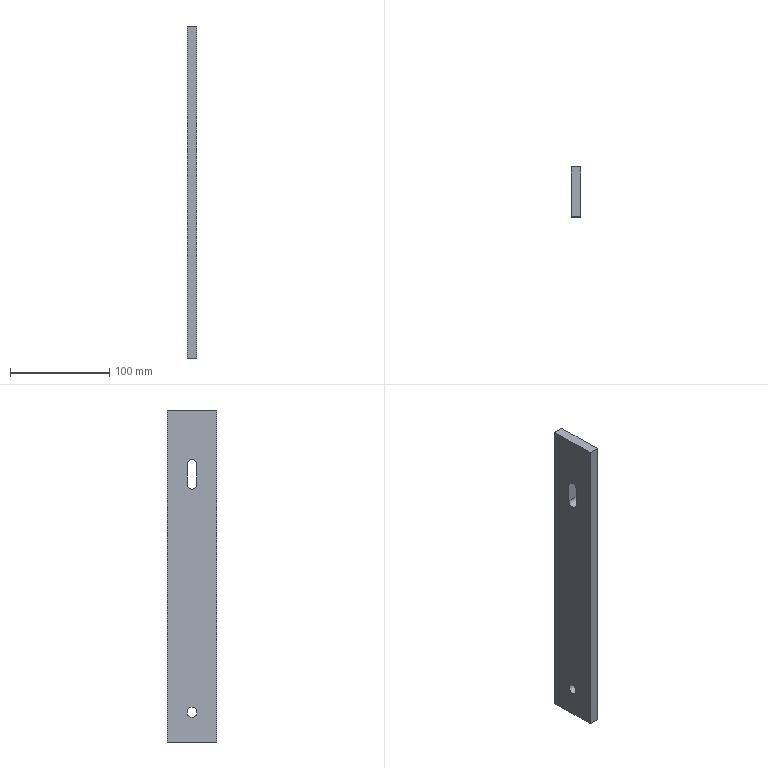Part | NX | features solid 2 | 1 solid | 11 faces | box 10 x 50 x 335 mm | volume 163929 mm3 | plane 8 | cylinder 3 | commonest cylinder face diameters 10 x3
STEP:
#1=CARTESIAN_POINT('',(-1445.,530.,70.));
#2=VERTEX_POINT('',#1);
#3=CARTESIAN_POINT('',(-1455.,530.,70.));
#4=VERTEX_POINT('',#3);
#5=CARTESIAN_POINT('',(-1445.,530.,70.));
#6=DIRECTION('',(1.,0.,0.));
#7=VECTOR('',#6,1000.);
#8=LINE('',#5,#7);
#9=EDGE_CURVE('',#2,#4,#8,.F.);
#10=ORIENTED_EDGE('',*,*,#9,.T.);
#11=CARTESIAN_POINT('',(-1455.,480.,70.));
#12=VERTEX_POINT('',#11);
#13=CARTESIAN_POINT('',(-1455.,530.,70.));
#14=DIRECTION('',(0.,-1.,0.));
#15=VECTOR('',#14,1000.);
#16=LINE('',#13,#15);
#17=EDGE_CURVE('',#4,#12,#16,.T.);
#18=ORIENTED_EDGE('',*,*,#17,.T.);
#19=CARTESIAN_POINT('',(-1445.,480.,70.));
#20=VERTEX_POINT('',#19);
#21=CARTESIAN_POINT('',(-1445.,480.,70.));
#22=DIRECTION('',(-1.,0.,0.));
#23=VECTOR('',#22,1000.);
#24=LINE('',#21,#23);
#25=EDGE_CURVE('',#20,#12,#24,.T.);
#26=ORIENTED_EDGE('',*,*,#25,.F.);
#27=CARTESIAN_POINT('',(-1445.,530.,70.));
#28=DIRECTION('',(0.,-1.,0.));
#29=VECTOR('',#28,1000.);
#30=LINE('',#27,#29);
#31=EDGE_CURVE('',#2,#20,#30,.T.);
#32=ORIENTED_EDGE('',*,*,#31,.F.);
#33=EDGE_LOOP('',(#10,#18,#26,#32));
#34=FACE_BOUND('',#33,.T.);
#35=CARTESIAN_POINT('',(-1445.,530.,70.));
#36=DIRECTION('',(0.,0.,1.));
#37=DIRECTION('',(0.,-1.,0.));
#38=AXIS2_PLACEMENT_3D('',#35,#36,#37);
#39=PLANE('',#38);
#40=ADVANCED_FACE('',(#34),#39,.T.);
#41=ORIENTED_EDGE('',*,*,#25,.T.);
#42=CARTESIAN_POINT('',(-1455.,480.,-265.));
#43=VERTEX_POINT('',#42);
#44=CARTESIAN_POINT('',(-1455.,480.,55.));
#45=DIRECTION('',(0.,0.,1.));
#46=VECTOR('',#45,1000.);
#47=LINE('',#44,#46);
#48=EDGE_CURVE('',#12,#43,#47,.F.);
#49=ORIENTED_EDGE('',*,*,#48,.T.);
#50=CARTESIAN_POINT('',(-1445.,480.,-265.));
#51=VERTEX_POINT('',#50);
#52=CARTESIAN_POINT('',(-1445.,480.,-265.));
#53=DIRECTION('',(-1.,0.,0.));
#54=VECTOR('',#53,1000.);
#55=LINE('',#52,#54);
#56=EDGE_CURVE('',#51,#43,#55,.T.);
#57=ORIENTED_EDGE('',*,*,#56,.F.);
#58=CARTESIAN_POINT('',(-1445.,480.,55.));
#59=DIRECTION('',(0.,0.,-1.));
#60=VECTOR('',#59,1000.);
#61=LINE('',#58,#60);
#62=EDGE_CURVE('',#20,#51,#61,.T.);
#63=ORIENTED_EDGE('',*,*,#62,.F.);
#64=EDGE_LOOP('',(#41,#49,#57,#63));
#65=FACE_BOUND('',#64,.T.);
#66=CARTESIAN_POINT('',(-1445.,480.,55.));
#67=DIRECTION('',(0.,-1.,0.));
#68=DIRECTION('',(0.,0.,-1.));
#69=AXIS2_PLACEMENT_3D('',#66,#67,#68);
#70=PLANE('',#69);
#71=ADVANCED_FACE('',(#65),#70,.T.);
#72=ORIENTED_EDGE('',*,*,#56,.T.);
#73=CARTESIAN_POINT('',(-1455.,530.,-265.));
#74=VERTEX_POINT('',#73);
#75=CARTESIAN_POINT('',(-1455.,530.,-265.));
#76=DIRECTION('',(0.,-1.,0.));
#77=VECTOR('',#76,1000.);
#78=LINE('',#75,#77);
#79=EDGE_CURVE('',#74,#43,#78,.T.);
#80=ORIENTED_EDGE('',*,*,#79,.F.);
#81=CARTESIAN_POINT('',(-1445.,530.,-265.));
#82=VERTEX_POINT('',#81);
#83=CARTESIAN_POINT('',(-1445.,530.,-265.));
#84=DIRECTION('',(-1.,0.,0.));
#85=VECTOR('',#84,1000.);
#86=LINE('',#83,#85);
#87=EDGE_CURVE('',#82,#74,#86,.T.);
#88=ORIENTED_EDGE('',*,*,#87,.F.);
#89=CARTESIAN_POINT('',(-1445.,530.,-265.));
#90=DIRECTION('',(0.,-1.,0.));
#91=VECTOR('',#90,1000.);
#92=LINE('',#89,#91);
#93=EDGE_CURVE('',#82,#51,#92,.T.);
#94=ORIENTED_EDGE('',*,*,#93,.T.);
#95=EDGE_LOOP('',(#72,#80,#88,#94));
#96=FACE_BOUND('',#95,.T.);
#97=CARTESIAN_POINT('',(-1445.,530.,-265.));
#98=DIRECTION('',(0.,0.,1.));
#99=DIRECTION('',(0.,-1.,0.));
#100=AXIS2_PLACEMENT_3D('',#97,#98,#99);
#101=PLANE('',#100);
#102=ADVANCED_FACE('',(#96),#101,.F.);
#103=CARTESIAN_POINT('',(-1445.,530.,55.));
#104=DIRECTION('',(0.,0.,-1.));
#105=VECTOR('',#104,1000.);
#106=LINE('',#103,#105);
#107=EDGE_CURVE('',#2,#82,#106,.T.);
#108=ORIENTED_EDGE('',*,*,#107,.T.);
#109=ORIENTED_EDGE('',*,*,#87,.T.);
#110=CARTESIAN_POINT('',(-1455.,530.,55.));
#111=DIRECTION('',(0.,0.,1.));
#112=VECTOR('',#111,1000.);
#113=LINE('',#110,#112);
#114=EDGE_CURVE('',#4,#74,#113,.F.);
#115=ORIENTED_EDGE('',*,*,#114,.F.);
#116=ORIENTED_EDGE('',*,*,#9,.F.);
#117=EDGE_LOOP('',(#108,#109,#115,#116));
#118=FACE_BOUND('',#117,.T.);
#119=CARTESIAN_POINT('',(-1445.,530.,55.));
#120=DIRECTION('',(0.,-1.,0.));
#121=DIRECTION('',(0.,0.,-1.));
#122=AXIS2_PLACEMENT_3D('',#119,#120,#121);
#123=PLANE('',#122);
#124=ADVANCED_FACE('',(#118),#123,.F.);
#125=CARTESIAN_POINT('',(-1455.,505.,-230.));
#126=VERTEX_POINT('',#125);
#127=CARTESIAN_POINT('',(-1455.,505.,-235.));
#128=DIRECTION('',(1.,0.,0.));
#129=DIRECTION('',(0.,0.,1.));
#130=AXIS2_PLACEMENT_3D('',#127,#128,#129);
#131=CIRCLE('',#130,5.);
#132=EDGE_CURVE('',#126,#126,#131,.T.);
#133=ORIENTED_EDGE('',*,*,#132,.T.);
#134=EDGE_LOOP('',(#133));
#135=FACE_BOUND('',#134,.T.);
#136=CARTESIAN_POINT('',(-1455.,510.,15.));
#137=VERTEX_POINT('',#136);
#138=CARTESIAN_POINT('',(-1455.,500.,15.));
#139=VERTEX_POINT('',#138);
#140=CARTESIAN_POINT('',(-1455.,505.,15.));
#141=DIRECTION('',(1.,0.,0.));
#142=DIRECTION('',(0.,0.,1.));
#143=AXIS2_PLACEMENT_3D('',#140,#141,#142);
#144=CIRCLE('',#143,5.);
#145=EDGE_CURVE('',#137,#139,#144,.T.);
#146=ORIENTED_EDGE('',*,*,#145,.T.);
#147=CARTESIAN_POINT('',(-1455.,500.,-5.));
#148=VERTEX_POINT('',#147);
#149=CARTESIAN_POINT('',(-1455.,500.,55.));
#150=DIRECTION('',(0.,0.,1.));
#151=VECTOR('',#150,1000.);
#152=LINE('',#149,#151);
#153=EDGE_CURVE('',#148,#139,#152,.T.);
#154=ORIENTED_EDGE('',*,*,#153,.F.);
#155=CARTESIAN_POINT('',(-1455.,510.,-5.));
#156=VERTEX_POINT('',#155);
#157=CARTESIAN_POINT('',(-1455.,505.,-5.));
#158=DIRECTION('',(1.,0.,0.));
#159=DIRECTION('',(0.,0.,1.));
#160=AXIS2_PLACEMENT_3D('',#157,#158,#159);
#161=CIRCLE('',#160,5.);
#162=EDGE_CURVE('',#148,#156,#161,.T.);
#163=ORIENTED_EDGE('',*,*,#162,.T.);
#164=CARTESIAN_POINT('',(-1455.,510.,55.));
#165=DIRECTION('',(0.,0.,1.));
#166=VECTOR('',#165,1000.);
#167=LINE('',#164,#166);
#168=EDGE_CURVE('',#156,#137,#167,.T.);
#169=ORIENTED_EDGE('',*,*,#168,.T.);
#170=EDGE_LOOP('',(#146,#154,#163,#169));
#171=FACE_BOUND('',#170,.T.);
#172=ORIENTED_EDGE('',*,*,#79,.T.);
#173=ORIENTED_EDGE('',*,*,#48,.F.);
#174=ORIENTED_EDGE('',*,*,#17,.F.);
#175=ORIENTED_EDGE('',*,*,#114,.T.);
#176=EDGE_LOOP('',(#172,#173,#174,#175));
#177=FACE_BOUND('',#176,.T.);
#178=CARTESIAN_POINT('',(-1455.,530.,55.));
#179=DIRECTION('',(-1.,0.,0.));
#180=DIRECTION('',(0.,0.,1.));
#181=AXIS2_PLACEMENT_3D('',#178,#179,#180);
#182=PLANE('',#181);
#183=ADVANCED_FACE('',(#135,#171,#177),#182,.T.);
#184=CARTESIAN_POINT('',(-1445.,505.,-230.));
#185=VERTEX_POINT('',#184);
#186=CARTESIAN_POINT('',(-1445.,505.,-235.));
#187=DIRECTION('',(1.,0.,0.));
#188=DIRECTION('',(0.,0.,1.));
#189=AXIS2_PLACEMENT_3D('',#186,#187,#188);
#190=CIRCLE('',#189,5.);
#191=EDGE_CURVE('',#185,#185,#190,.T.);
#192=ORIENTED_EDGE('',*,*,#191,.F.);
#193=EDGE_LOOP('',(#192));
#194=FACE_BOUND('',#193,.T.);
#195=CARTESIAN_POINT('',(-1445.,510.,-5.));
#196=VERTEX_POINT('',#195);
#197=CARTESIAN_POINT('',(-1445.,510.,15.));
#198=VERTEX_POINT('',#197);
#199=CARTESIAN_POINT('',(-1445.,510.,55.));
#200=DIRECTION('',(0.,0.,1.));
#201=VECTOR('',#200,1000.);
#202=LINE('',#199,#201);
#203=EDGE_CURVE('',#196,#198,#202,.T.);
#204=ORIENTED_EDGE('',*,*,#203,.F.);
#205=CARTESIAN_POINT('',(-1445.,500.,-5.));
#206=VERTEX_POINT('',#205);
#207=CARTESIAN_POINT('',(-1445.,505.,-5.));
#208=DIRECTION('',(1.,0.,0.));
#209=DIRECTION('',(0.,0.,1.));
#210=AXIS2_PLACEMENT_3D('',#207,#208,#209);
#211=CIRCLE('',#210,5.);
#212=EDGE_CURVE('',#206,#196,#211,.T.);
#213=ORIENTED_EDGE('',*,*,#212,.F.);
#214=CARTESIAN_POINT('',(-1445.,500.,15.));
#215=VERTEX_POINT('',#214);
#216=CARTESIAN_POINT('',(-1445.,500.,55.));
#217=DIRECTION('',(0.,0.,1.));
#218=VECTOR('',#217,1000.);
#219=LINE('',#216,#218);
#220=EDGE_CURVE('',#206,#215,#219,.T.);
#221=ORIENTED_EDGE('',*,*,#220,.T.);
#222=CARTESIAN_POINT('',(-1445.,505.,15.));
#223=DIRECTION('',(1.,0.,0.));
#224=DIRECTION('',(0.,0.,1.));
#225=AXIS2_PLACEMENT_3D('',#222,#223,#224);
#226=CIRCLE('',#225,5.);
#227=EDGE_CURVE('',#198,#215,#226,.T.);
#228=ORIENTED_EDGE('',*,*,#227,.F.);
#229=EDGE_LOOP('',(#204,#213,#221,#228));
#230=FACE_BOUND('',#229,.T.);
#231=ORIENTED_EDGE('',*,*,#93,.F.);
#232=ORIENTED_EDGE('',*,*,#107,.F.);
#233=ORIENTED_EDGE('',*,*,#31,.T.);
#234=ORIENTED_EDGE('',*,*,#62,.T.);
#235=EDGE_LOOP('',(#231,#232,#233,#234));
#236=FACE_BOUND('',#235,.T.);
#237=CARTESIAN_POINT('',(-1445.,530.,55.));
#238=DIRECTION('',(-1.,0.,0.));
#239=DIRECTION('',(0.,0.,1.));
#240=AXIS2_PLACEMENT_3D('',#237,#238,#239);
#241=PLANE('',#240);
#242=ADVANCED_FACE('',(#194,#230,#236),#241,.F.);
#243=ORIENTED_EDGE('',*,*,#145,.F.);
#244=CARTESIAN_POINT('',(-1505.,510.,15.));
#245=DIRECTION('',(1.,0.,0.));
#246=VECTOR('',#245,1000.);
#247=LINE('',#244,#246);
#248=EDGE_CURVE('',#137,#198,#247,.T.);
#249=ORIENTED_EDGE('',*,*,#248,.T.);
#250=ORIENTED_EDGE('',*,*,#227,.T.);
#251=CARTESIAN_POINT('',(-1505.,500.,15.));
#252=DIRECTION('',(1.,0.,0.));
#253=VECTOR('',#252,1000.);
#254=LINE('',#251,#253);
#255=EDGE_CURVE('',#139,#215,#254,.T.);
#256=ORIENTED_EDGE('',*,*,#255,.F.);
#257=EDGE_LOOP('',(#243,#249,#250,#256));
#258=FACE_BOUND('',#257,.T.);
#259=CARTESIAN_POINT('',(-1505.,505.,15.));
#260=DIRECTION('',(1.,0.,0.));
#261=DIRECTION('',(0.,0.,-1.));
#262=AXIS2_PLACEMENT_3D('',#259,#260,#261);
#263=CYLINDRICAL_SURFACE('',#262,5.);
#264=ADVANCED_FACE('',(#258),#263,.F.);
#265=ORIENTED_EDGE('',*,*,#168,.F.);
#266=CARTESIAN_POINT('',(-1505.,510.,-5.));
#267=DIRECTION('',(1.,0.,0.));
#268=VECTOR('',#267,1000.);
#269=LINE('',#266,#268);
#270=EDGE_CURVE('',#156,#196,#269,.T.);
#271=ORIENTED_EDGE('',*,*,#270,.T.);
#272=ORIENTED_EDGE('',*,*,#203,.T.);
#273=ORIENTED_EDGE('',*,*,#248,.F.);
#274=EDGE_LOOP('',(#265,#271,#272,#273));
#275=FACE_BOUND('',#274,.T.);
#276=CARTESIAN_POINT('',(-1505.,510.,15.));
#277=DIRECTION('',(0.,1.,0.));
#278=DIRECTION('',(0.,0.,1.));
#279=AXIS2_PLACEMENT_3D('',#276,#277,#278);
#280=PLANE('',#279);
#281=ADVANCED_FACE('',(#275),#280,.F.);
#282=ORIENTED_EDGE('',*,*,#162,.F.);
#283=CARTESIAN_POINT('',(-1505.,500.,-5.));
#284=DIRECTION('',(1.,0.,0.));
#285=VECTOR('',#284,1000.);
#286=LINE('',#283,#285);
#287=EDGE_CURVE('',#148,#206,#286,.T.);
#288=ORIENTED_EDGE('',*,*,#287,.T.);
#289=ORIENTED_EDGE('',*,*,#212,.T.);
#290=ORIENTED_EDGE('',*,*,#270,.F.);
#291=EDGE_LOOP('',(#282,#288,#289,#290));
#292=FACE_BOUND('',#291,.T.);
#293=CARTESIAN_POINT('',(-1505.,505.,-5.));
#294=DIRECTION('',(1.,0.,0.));
#295=DIRECTION('',(0.,0.,-1.));
#296=AXIS2_PLACEMENT_3D('',#293,#294,#295);
#297=CYLINDRICAL_SURFACE('',#296,5.);
#298=ADVANCED_FACE('',(#292),#297,.F.);
#299=ORIENTED_EDGE('',*,*,#287,.F.);
#300=ORIENTED_EDGE('',*,*,#153,.T.);
#301=ORIENTED_EDGE('',*,*,#255,.T.);
#302=ORIENTED_EDGE('',*,*,#220,.F.);
#303=EDGE_LOOP('',(#299,#300,#301,#302));
#304=FACE_BOUND('',#303,.T.);
#305=CARTESIAN_POINT('',(-1505.,500.,15.));
#306=DIRECTION('',(0.,1.,0.));
#307=DIRECTION('',(0.,0.,1.));
#308=AXIS2_PLACEMENT_3D('',#305,#306,#307);
#309=PLANE('',#308);
#310=ADVANCED_FACE('',(#304),#309,.T.);
#311=ORIENTED_EDGE('',*,*,#132,.F.);
#312=EDGE_LOOP('',(#311));
#313=FACE_BOUND('',#312,.T.);
#314=ORIENTED_EDGE('',*,*,#191,.T.);
#315=EDGE_LOOP('',(#314));
#316=FACE_BOUND('',#315,.T.);
#317=CARTESIAN_POINT('',(-1505.,505.,-235.));
#318=DIRECTION('',(1.,0.,0.));
#319=DIRECTION('',(0.,0.,-1.));
#320=AXIS2_PLACEMENT_3D('',#317,#318,#319);
#321=CYLINDRICAL_SURFACE('',#320,5.);
#322=ADVANCED_FACE('',(#313,#316),#321,.F.);
#323=CLOSED_SHELL('',(#40,#71,#102,#124,#183,#242,#264,#281,#298,#310,#322));
#324=MANIFOLD_SOLID_BREP('',#323);
#325=(LENGTH_UNIT()NAMED_UNIT(*)SI_UNIT(.MILLI.,.METRE.));
#326=UNCERTAINTY_MEASURE_WITH_UNIT(LENGTH_MEASURE(0.00001),#325,'','');
#327=(NAMED_UNIT(*)PLANE_ANGLE_UNIT()SI_UNIT($,.RADIAN.));
#328=(NAMED_UNIT(*)SI_UNIT($,.STERADIAN.)SOLID_ANGLE_UNIT());
#329=(GEOMETRIC_REPRESENTATION_CONTEXT(3)GLOBAL_UNCERTAINTY_ASSIGNED_CONTEXT((#326))GLOBAL_UNIT_ASSIGNED_CONTEXT((#325,#327,#328))REPRESENTATION_CONTEXT('',''));
#330=ADVANCED_BREP_SHAPE_REPRESENTATION('',(#324),#329);